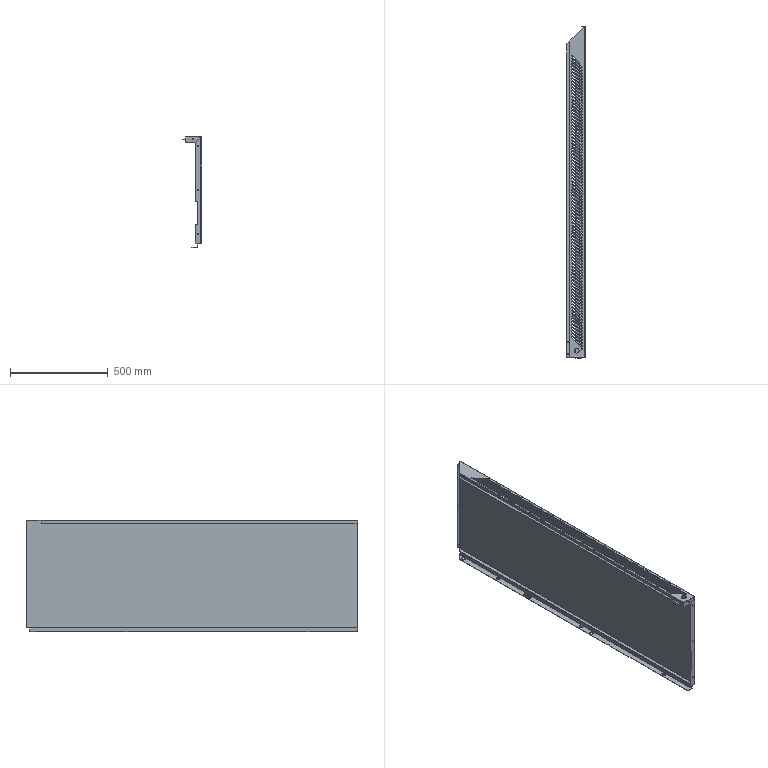Part | STEP file | HESS-408-70-15W-D-2-electrical box right side panel | 1 solid | 629 faces | box 93.5 x 1699 x 568.5 mm | volume 1802522 mm3 | cylinder 366 | plane 257 | spline 6 | commonest cylinder face diameters 5 x291 3.2 x15 5.5 x14 6 x11 0.2 x9 15 x9